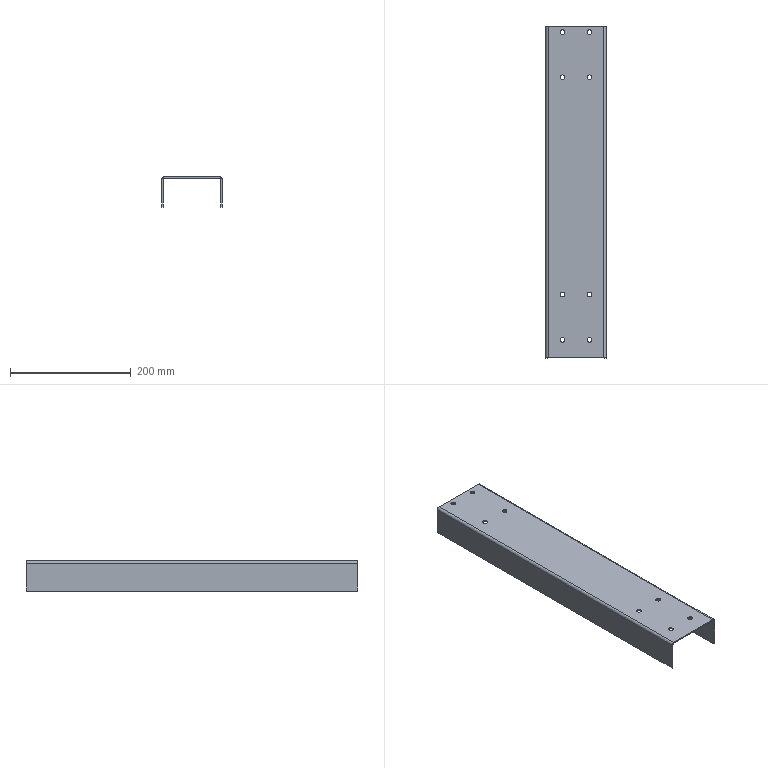Part | SolidWorks | features EdgeFlange 1, FlatPattern 1, ICE 1, SMBaseFlange 1, SheetMetal 1 | 1 solid | 38 faces | box 100 x 550 x 50 mm | volume 211963 mm3 | cylinder 20 | plane 18 | commonest cylinder face diameters 8 x18 4 x2
STEP:
#1=CARTESIAN_POINT('',(12.564,-446.02,-2.));
#2=VERTEX_POINT('',#1);
#3=CARTESIAN_POINT('',(20.564,-446.02,-2.));
#4=VERTEX_POINT('',#3);
#5=CARTESIAN_POINT('',(16.564,-446.02,-2.));
#6=DIRECTION('',(0.,0.,1.));
#7=DIRECTION('',(1.,0.,0.));
#8=AXIS2_PLACEMENT_3D('',#5,#6,#7);
#9=CIRCLE('',#8,4.);
#10=EDGE_CURVE('',#2,#4,#9,.T.);
#11=ORIENTED_EDGE('',*,*,#10,.F.);
#12=CARTESIAN_POINT('',(12.564,-446.02,0.));
#13=VERTEX_POINT('',#12);
#14=CARTESIAN_POINT('',(12.564,-446.02,-10.));
#15=DIRECTION('',(0.,0.,1.));
#16=VECTOR('',#15,1000.);
#17=LINE('',#14,#16);
#18=EDGE_CURVE('',#2,#13,#17,.T.);
#19=ORIENTED_EDGE('',*,*,#18,.T.);
#20=CARTESIAN_POINT('',(20.564,-446.02,0.));
#21=VERTEX_POINT('',#20);
#22=CARTESIAN_POINT('',(16.564,-446.02,0.));
#23=DIRECTION('',(0.,0.,1.));
#24=DIRECTION('',(-1.,0.,0.));
#25=AXIS2_PLACEMENT_3D('',#22,#23,#24);
#26=CIRCLE('',#25,4.);
#27=EDGE_CURVE('',#13,#21,#26,.T.);
#28=ORIENTED_EDGE('',*,*,#27,.T.);
#29=CARTESIAN_POINT('',(20.564,-446.02,-10.));
#30=DIRECTION('',(0.,0.,1.));
#31=VECTOR('',#30,1000.);
#32=LINE('',#29,#31);
#33=EDGE_CURVE('',#4,#21,#32,.T.);
#34=ORIENTED_EDGE('',*,*,#33,.F.);
#35=EDGE_LOOP('',(#11,#19,#28,#34));
#36=FACE_OUTER_BOUND('',#35,.T.);
#37=CARTESIAN_POINT('',(16.564,-446.02,-10.));
#38=DIRECTION('',(0.,0.,1.));
#39=DIRECTION('',(1.,0.,0.));
#40=AXIS2_PLACEMENT_3D('',#37,#38,#39);
#41=CYLINDRICAL_SURFACE('',#40,4.);
#42=ADVANCED_FACE('',(#36),#41,.F.);
#43=CARTESIAN_POINT('',(57.564,-446.02,-2.));
#44=VERTEX_POINT('',#43);
#45=CARTESIAN_POINT('',(65.564,-446.02,-2.));
#46=VERTEX_POINT('',#45);
#47=CARTESIAN_POINT('',(61.564,-446.02,-2.));
#48=DIRECTION('',(0.,0.,1.));
#49=DIRECTION('',(1.,0.,0.));
#50=AXIS2_PLACEMENT_3D('',#47,#48,#49);
#51=CIRCLE('',#50,4.);
#52=EDGE_CURVE('',#44,#46,#51,.T.);
#53=ORIENTED_EDGE('',*,*,#52,.F.);
#54=CARTESIAN_POINT('',(57.564,-446.02,0.));
#55=VERTEX_POINT('',#54);
#56=CARTESIAN_POINT('',(57.564,-446.02,-10.));
#57=DIRECTION('',(0.,0.,1.));
#58=VECTOR('',#57,1000.);
#59=LINE('',#56,#58);
#60=EDGE_CURVE('',#44,#55,#59,.T.);
#61=ORIENTED_EDGE('',*,*,#60,.T.);
#62=CARTESIAN_POINT('',(65.564,-446.02,0.));
#63=VERTEX_POINT('',#62);
#64=CARTESIAN_POINT('',(61.564,-446.02,0.));
#65=DIRECTION('',(0.,0.,1.));
#66=DIRECTION('',(-1.,0.,0.));
#67=AXIS2_PLACEMENT_3D('',#64,#65,#66);
#68=CIRCLE('',#67,4.);
#69=EDGE_CURVE('',#55,#63,#68,.T.);
#70=ORIENTED_EDGE('',*,*,#69,.T.);
#71=CARTESIAN_POINT('',(65.564,-446.02,-10.));
#72=DIRECTION('',(0.,0.,1.));
#73=VECTOR('',#72,1000.);
#74=LINE('',#71,#73);
#75=EDGE_CURVE('',#46,#63,#74,.T.);
#76=ORIENTED_EDGE('',*,*,#75,.F.);
#77=EDGE_LOOP('',(#53,#61,#70,#76));
#78=FACE_OUTER_BOUND('',#77,.T.);
#79=CARTESIAN_POINT('',(61.564,-446.02,-10.));
#80=DIRECTION('',(0.,0.,1.));
#81=DIRECTION('',(1.,0.,0.));
#82=AXIS2_PLACEMENT_3D('',#79,#80,#81);
#83=CYLINDRICAL_SURFACE('',#82,4.);
#84=ADVANCED_FACE('',(#78),#83,.F.);
#85=CARTESIAN_POINT('',(12.564,-371.02,-2.));
#86=VERTEX_POINT('',#85);
#87=CARTESIAN_POINT('',(20.564,-371.02,-2.));
#88=VERTEX_POINT('',#87);
#89=CARTESIAN_POINT('',(16.564,-371.02,-2.));
#90=DIRECTION('',(0.,0.,1.));
#91=DIRECTION('',(1.,0.,0.));
#92=AXIS2_PLACEMENT_3D('',#89,#90,#91);
#93=CIRCLE('',#92,4.);
#94=EDGE_CURVE('',#86,#88,#93,.T.);
#95=ORIENTED_EDGE('',*,*,#94,.F.);
#96=CARTESIAN_POINT('',(12.564,-371.02,0.));
#97=VERTEX_POINT('',#96);
#98=CARTESIAN_POINT('',(12.564,-371.02,-10.));
#99=DIRECTION('',(0.,0.,1.));
#100=VECTOR('',#99,1000.);
#101=LINE('',#98,#100);
#102=EDGE_CURVE('',#86,#97,#101,.T.);
#103=ORIENTED_EDGE('',*,*,#102,.T.);
#104=CARTESIAN_POINT('',(20.564,-371.02,0.));
#105=VERTEX_POINT('',#104);
#106=CARTESIAN_POINT('',(16.564,-371.02,0.));
#107=DIRECTION('',(0.,0.,1.));
#108=DIRECTION('',(-1.,0.,0.));
#109=AXIS2_PLACEMENT_3D('',#106,#107,#108);
#110=CIRCLE('',#109,4.);
#111=EDGE_CURVE('',#97,#105,#110,.T.);
#112=ORIENTED_EDGE('',*,*,#111,.T.);
#113=CARTESIAN_POINT('',(20.564,-371.02,-10.));
#114=DIRECTION('',(0.,0.,1.));
#115=VECTOR('',#114,1000.);
#116=LINE('',#113,#115);
#117=EDGE_CURVE('',#88,#105,#116,.T.);
#118=ORIENTED_EDGE('',*,*,#117,.F.);
#119=EDGE_LOOP('',(#95,#103,#112,#118));
#120=FACE_OUTER_BOUND('',#119,.T.);
#121=CARTESIAN_POINT('',(16.564,-371.02,-10.));
#122=DIRECTION('',(0.,0.,1.));
#123=DIRECTION('',(1.,0.,0.));
#124=AXIS2_PLACEMENT_3D('',#121,#122,#123);
#125=CYLINDRICAL_SURFACE('',#124,4.);
#126=ADVANCED_FACE('',(#120),#125,.F.);
#127=CARTESIAN_POINT('',(57.564,-371.02,-2.));
#128=VERTEX_POINT('',#127);
#129=CARTESIAN_POINT('',(65.564,-371.02,-2.));
#130=VERTEX_POINT('',#129);
#131=CARTESIAN_POINT('',(61.564,-371.02,-2.));
#132=DIRECTION('',(0.,0.,1.));
#133=DIRECTION('',(1.,0.,0.));
#134=AXIS2_PLACEMENT_3D('',#131,#132,#133);
#135=CIRCLE('',#134,4.);
#136=EDGE_CURVE('',#128,#130,#135,.T.);
#137=ORIENTED_EDGE('',*,*,#136,.F.);
#138=CARTESIAN_POINT('',(57.564,-371.02,0.));
#139=VERTEX_POINT('',#138);
#140=CARTESIAN_POINT('',(57.564,-371.02,-10.));
#141=DIRECTION('',(0.,0.,1.));
#142=VECTOR('',#141,1000.);
#143=LINE('',#140,#142);
#144=EDGE_CURVE('',#128,#139,#143,.T.);
#145=ORIENTED_EDGE('',*,*,#144,.T.);
#146=CARTESIAN_POINT('',(65.564,-371.02,0.));
#147=VERTEX_POINT('',#146);
#148=CARTESIAN_POINT('',(61.564,-371.02,0.));
#149=DIRECTION('',(0.,0.,1.));
#150=DIRECTION('',(-1.,0.,0.));
#151=AXIS2_PLACEMENT_3D('',#148,#149,#150);
#152=CIRCLE('',#151,4.);
#153=EDGE_CURVE('',#139,#147,#152,.T.);
#154=ORIENTED_EDGE('',*,*,#153,.T.);
#155=CARTESIAN_POINT('',(65.564,-371.02,-10.));
#156=DIRECTION('',(0.,0.,1.));
#157=VECTOR('',#156,1000.);
#158=LINE('',#155,#157);
#159=EDGE_CURVE('',#130,#147,#158,.T.);
#160=ORIENTED_EDGE('',*,*,#159,.F.);
#161=EDGE_LOOP('',(#137,#145,#154,#160));
#162=FACE_OUTER_BOUND('',#161,.T.);
#163=CARTESIAN_POINT('',(61.564,-371.02,-10.));
#164=DIRECTION('',(0.,0.,1.));
#165=DIRECTION('',(1.,0.,0.));
#166=AXIS2_PLACEMENT_3D('',#163,#164,#165);
#167=CYLINDRICAL_SURFACE('',#166,4.);
#168=ADVANCED_FACE('',(#162),#167,.F.);
#169=CARTESIAN_POINT('',(57.564,-11.02,-2.));
#170=VERTEX_POINT('',#169);
#171=CARTESIAN_POINT('',(65.564,-11.02,-2.));
#172=VERTEX_POINT('',#171);
#173=CARTESIAN_POINT('',(61.564,-11.02,-2.));
#174=DIRECTION('',(0.,0.,1.));
#175=DIRECTION('',(1.,0.,0.));
#176=AXIS2_PLACEMENT_3D('',#173,#174,#175);
#177=CIRCLE('',#176,4.);
#178=EDGE_CURVE('',#170,#172,#177,.T.);
#179=ORIENTED_EDGE('',*,*,#178,.F.);
#180=CARTESIAN_POINT('',(57.564,-11.02,0.));
#181=VERTEX_POINT('',#180);
#182=CARTESIAN_POINT('',(57.564,-11.02,-10.));
#183=DIRECTION('',(0.,0.,1.));
#184=VECTOR('',#183,1000.);
#185=LINE('',#182,#184);
#186=EDGE_CURVE('',#170,#181,#185,.T.);
#187=ORIENTED_EDGE('',*,*,#186,.T.);
#188=CARTESIAN_POINT('',(65.564,-11.02,0.));
#189=VERTEX_POINT('',#188);
#190=CARTESIAN_POINT('',(61.564,-11.02,0.));
#191=DIRECTION('',(0.,0.,1.));
#192=DIRECTION('',(1.,0.,0.));
#193=AXIS2_PLACEMENT_3D('',#190,#191,#192);
#194=CIRCLE('',#193,4.);
#195=EDGE_CURVE('',#181,#189,#194,.T.);
#196=ORIENTED_EDGE('',*,*,#195,.T.);
#197=CARTESIAN_POINT('',(65.564,-11.02,-10.));
#198=DIRECTION('',(0.,0.,1.));
#199=VECTOR('',#198,1000.);
#200=LINE('',#197,#199);
#201=EDGE_CURVE('',#172,#189,#200,.T.);
#202=ORIENTED_EDGE('',*,*,#201,.F.);
#203=EDGE_LOOP('',(#179,#187,#196,#202));
#204=FACE_OUTER_BOUND('',#203,.T.);
#205=CARTESIAN_POINT('',(61.564,-11.02,-10.));
#206=DIRECTION('',(0.,0.,1.));
#207=DIRECTION('',(1.,0.,0.));
#208=AXIS2_PLACEMENT_3D('',#205,#206,#207);
#209=CYLINDRICAL_SURFACE('',#208,4.);
#210=ADVANCED_FACE('',(#204),#209,.F.);
#211=CARTESIAN_POINT('',(12.564,-11.02,-2.));
#212=VERTEX_POINT('',#211);
#213=CARTESIAN_POINT('',(20.564,-11.02,-2.));
#214=VERTEX_POINT('',#213);
#215=CARTESIAN_POINT('',(16.564,-11.02,-2.));
#216=DIRECTION('',(0.,0.,1.));
#217=DIRECTION('',(1.,0.,0.));
#218=AXIS2_PLACEMENT_3D('',#215,#216,#217);
#219=CIRCLE('',#218,4.);
#220=EDGE_CURVE('',#212,#214,#219,.T.);
#221=ORIENTED_EDGE('',*,*,#220,.F.);
#222=CARTESIAN_POINT('',(12.564,-11.02,0.));
#223=VERTEX_POINT('',#222);
#224=CARTESIAN_POINT('',(12.564,-11.02,-10.));
#225=DIRECTION('',(0.,0.,1.));
#226=VECTOR('',#225,1000.);
#227=LINE('',#224,#226);
#228=EDGE_CURVE('',#212,#223,#227,.T.);
#229=ORIENTED_EDGE('',*,*,#228,.T.);
#230=CARTESIAN_POINT('',(20.564,-11.02,0.));
#231=VERTEX_POINT('',#230);
#232=CARTESIAN_POINT('',(16.564,-11.02,0.));
#233=DIRECTION('',(0.,0.,1.));
#234=DIRECTION('',(1.,0.,0.));
#235=AXIS2_PLACEMENT_3D('',#232,#233,#234);
#236=CIRCLE('',#235,4.);
#237=EDGE_CURVE('',#223,#231,#236,.T.);
#238=ORIENTED_EDGE('',*,*,#237,.T.);
#239=CARTESIAN_POINT('',(20.564,-11.02,-10.));
#240=DIRECTION('',(0.,0.,1.));
#241=VECTOR('',#240,1000.);
#242=LINE('',#239,#241);
#243=EDGE_CURVE('',#214,#231,#242,.T.);
#244=ORIENTED_EDGE('',*,*,#243,.F.);
#245=EDGE_LOOP('',(#221,#229,#238,#244));
#246=FACE_OUTER_BOUND('',#245,.T.);
#247=CARTESIAN_POINT('',(16.564,-11.02,-10.));
#248=DIRECTION('',(0.,0.,1.));
#249=DIRECTION('',(1.,0.,0.));
#250=AXIS2_PLACEMENT_3D('',#247,#248,#249);
#251=CYLINDRICAL_SURFACE('',#250,4.);
#252=ADVANCED_FACE('',(#246),#251,.F.);
#253=CARTESIAN_POINT('',(57.564,63.98,-2.));
#254=VERTEX_POINT('',#253);
#255=CARTESIAN_POINT('',(65.564,63.98,-2.));
#256=VERTEX_POINT('',#255);
#257=CARTESIAN_POINT('',(61.564,63.98,-2.));
#258=DIRECTION('',(0.,0.,1.));
#259=DIRECTION('',(1.,0.,0.));
#260=AXIS2_PLACEMENT_3D('',#257,#258,#259);
#261=CIRCLE('',#260,4.);
#262=EDGE_CURVE('',#254,#256,#261,.T.);
#263=ORIENTED_EDGE('',*,*,#262,.F.);
#264=CARTESIAN_POINT('',(57.564,63.98,0.));
#265=VERTEX_POINT('',#264);
#266=CARTESIAN_POINT('',(57.564,63.98,-10.));
#267=DIRECTION('',(0.,0.,1.));
#268=VECTOR('',#267,1000.);
#269=LINE('',#266,#268);
#270=EDGE_CURVE('',#254,#265,#269,.T.);
#271=ORIENTED_EDGE('',*,*,#270,.T.);
#272=CARTESIAN_POINT('',(65.564,63.98,0.));
#273=VERTEX_POINT('',#272);
#274=CARTESIAN_POINT('',(61.564,63.98,0.));
#275=DIRECTION('',(0.,0.,1.));
#276=DIRECTION('',(1.,0.,0.));
#277=AXIS2_PLACEMENT_3D('',#274,#275,#276);
#278=CIRCLE('',#277,4.);
#279=EDGE_CURVE('',#265,#273,#278,.T.);
#280=ORIENTED_EDGE('',*,*,#279,.T.);
#281=CARTESIAN_POINT('',(65.564,63.98,-10.));
#282=DIRECTION('',(0.,0.,1.));
#283=VECTOR('',#282,1000.);
#284=LINE('',#281,#283);
#285=EDGE_CURVE('',#256,#273,#284,.T.);
#286=ORIENTED_EDGE('',*,*,#285,.F.);
#287=EDGE_LOOP('',(#263,#271,#280,#286));
#288=FACE_OUTER_BOUND('',#287,.T.);
#289=CARTESIAN_POINT('',(61.564,63.98,-10.));
#290=DIRECTION('',(0.,0.,1.));
#291=DIRECTION('',(1.,0.,0.));
#292=AXIS2_PLACEMENT_3D('',#289,#290,#291);
#293=CYLINDRICAL_SURFACE('',#292,4.);
#294=ADVANCED_FACE('',(#288),#293,.F.);
#295=CARTESIAN_POINT('',(12.564,63.98,-2.));
#296=VERTEX_POINT('',#295);
#297=CARTESIAN_POINT('',(20.564,63.98,-2.));
#298=VERTEX_POINT('',#297);
#299=CARTESIAN_POINT('',(16.564,63.98,-2.));
#300=DIRECTION('',(0.,0.,1.));
#301=DIRECTION('',(1.,0.,0.));
#302=AXIS2_PLACEMENT_3D('',#299,#300,#301);
#303=CIRCLE('',#302,4.);
#304=EDGE_CURVE('',#296,#298,#303,.T.);
#305=ORIENTED_EDGE('',*,*,#304,.F.);
#306=CARTESIAN_POINT('',(12.564,63.98,0.));
#307=VERTEX_POINT('',#306);
#308=CARTESIAN_POINT('',(12.564,63.98,-10.));
#309=DIRECTION('',(0.,0.,1.));
#310=VECTOR('',#309,1000.);
#311=LINE('',#308,#310);
#312=EDGE_CURVE('',#296,#307,#311,.T.);
#313=ORIENTED_EDGE('',*,*,#312,.T.);
#314=CARTESIAN_POINT('',(20.564,63.98,0.));
#315=VERTEX_POINT('',#314);
#316=CARTESIAN_POINT('',(16.564,63.98,0.));
#317=DIRECTION('',(0.,0.,1.));
#318=DIRECTION('',(1.,0.,0.));
#319=AXIS2_PLACEMENT_3D('',#316,#317,#318);
#320=CIRCLE('',#319,4.);
#321=EDGE_CURVE('',#307,#315,#320,.T.);
#322=ORIENTED_EDGE('',*,*,#321,.T.);
#323=CARTESIAN_POINT('',(20.564,63.98,-10.));
#324=DIRECTION('',(0.,0.,1.));
#325=VECTOR('',#324,1000.);
#326=LINE('',#323,#325);
#327=EDGE_CURVE('',#298,#315,#326,.T.);
#328=ORIENTED_EDGE('',*,*,#327,.F.);
#329=EDGE_LOOP('',(#305,#313,#322,#328));
#330=FACE_OUTER_BOUND('',#329,.T.);
#331=CARTESIAN_POINT('',(16.564,63.98,-10.));
#332=DIRECTION('',(0.,0.,1.));
#333=DIRECTION('',(1.,0.,0.));
#334=AXIS2_PLACEMENT_3D('',#331,#332,#333);
#335=CYLINDRICAL_SURFACE('',#334,4.);
#336=ADVANCED_FACE('',(#330),#335,.F.);
#337=CARTESIAN_POINT('',(16.564,-446.02,-2.));
#338=DIRECTION('',(0.,0.,1.));
#339=DIRECTION('',(1.,0.,0.));
#340=AXIS2_PLACEMENT_3D('',#337,#338,#339);
#341=CIRCLE('',#340,4.);
#342=EDGE_CURVE('',#4,#2,#341,.T.);
#343=ORIENTED_EDGE('',*,*,#342,.T.);
#344=ORIENTED_EDGE('',*,*,#10,.T.);
#345=EDGE_LOOP('',(#343,#344));
#346=FACE_BOUND('',#345,.T.);
#347=CARTESIAN_POINT('',(61.564,-446.02,-2.));
#348=DIRECTION('',(0.,0.,1.));
#349=DIRECTION('',(1.,0.,0.));
#350=AXIS2_PLACEMENT_3D('',#347,#348,#349);
#351=CIRCLE('',#350,4.);
#352=EDGE_CURVE('',#46,#44,#351,.T.);
#353=ORIENTED_EDGE('',*,*,#352,.T.);
#354=ORIENTED_EDGE('',*,*,#52,.T.);
#355=EDGE_LOOP('',(#353,#354));
#356=FACE_BOUND('',#355,.T.);
#357=CARTESIAN_POINT('',(16.564,-371.02,-2.));
#358=DIRECTION('',(0.,0.,1.));
#359=DIRECTION('',(1.,0.,0.));
#360=AXIS2_PLACEMENT_3D('',#357,#358,#359);
#361=CIRCLE('',#360,4.);
#362=EDGE_CURVE('',#88,#86,#361,.T.);
#363=ORIENTED_EDGE('',*,*,#362,.T.);
#364=ORIENTED_EDGE('',*,*,#94,.T.);
#365=EDGE_LOOP('',(#363,#364));
#366=FACE_BOUND('',#365,.T.);
#367=CARTESIAN_POINT('',(61.564,-371.02,-2.));
#368=DIRECTION('',(0.,0.,1.));
#369=DIRECTION('',(1.,0.,0.));
#370=AXIS2_PLACEMENT_3D('',#367,#368,#369);
#371=CIRCLE('',#370,4.);
#372=EDGE_CURVE('',#130,#128,#371,.T.);
#373=ORIENTED_EDGE('',*,*,#372,.T.);
#374=ORIENTED_EDGE('',*,*,#136,.T.);
#375=EDGE_LOOP('',(#373,#374));
#376=FACE_BOUND('',#375,.T.);
#377=CARTESIAN_POINT('',(61.564,-11.02,-2.));
#378=DIRECTION('',(0.,0.,1.));
#379=DIRECTION('',(1.,0.,0.));
#380=AXIS2_PLACEMENT_3D('',#377,#378,#379);
#381=CIRCLE('',#380,4.);
#382=EDGE_CURVE('',#172,#170,#381,.T.);
#383=ORIENTED_EDGE('',*,*,#382,.T.);
#384=ORIENTED_EDGE('',*,*,#178,.T.);
#385=EDGE_LOOP('',(#383,#384));
#386=FACE_BOUND('',#385,.T.);
#387=CARTESIAN_POINT('',(16.564,-11.02,-2.));
#388=DIRECTION('',(0.,0.,1.));
#389=DIRECTION('',(1.,0.,0.));
#390=AXIS2_PLACEMENT_3D('',#387,#388,#389);
#391=CIRCLE('',#390,4.);
#392=EDGE_CURVE('',#214,#212,#391,.T.);
#393=ORIENTED_EDGE('',*,*,#392,.T.);
#394=ORIENTED_EDGE('',*,*,#220,.T.);
#395=EDGE_LOOP('',(#393,#394));
#396=FACE_BOUND('',#395,.T.);
#397=CARTESIAN_POINT('',(61.564,63.98,-2.));
#398=DIRECTION('',(0.,0.,1.));
#399=DIRECTION('',(1.,0.,0.));
#400=AXIS2_PLACEMENT_3D('',#397,#398,#399);
#401=CIRCLE('',#400,4.);
#402=EDGE_CURVE('',#256,#254,#401,.T.);
#403=ORIENTED_EDGE('',*,*,#402,.T.);
#404=ORIENTED_EDGE('',*,*,#262,.T.);
#405=EDGE_LOOP('',(#403,#404));
#406=FACE_BOUND('',#405,.T.);
#407=CARTESIAN_POINT('',(16.564,63.98,-2.));
#408=DIRECTION('',(0.,0.,1.));
#409=DIRECTION('',(1.,0.,0.));
#410=AXIS2_PLACEMENT_3D('',#407,#408,#409);
#411=CIRCLE('',#410,4.);
#412=EDGE_CURVE('',#298,#296,#411,.T.);
#413=ORIENTED_EDGE('',*,*,#412,.T.);
#414=ORIENTED_EDGE('',*,*,#304,.T.);
#415=EDGE_LOOP('',(#413,#414));
#416=FACE_BOUND('',#415,.T.);
#417=CARTESIAN_POINT('',(85.064,-476.02,-2.));
#418=VERTEX_POINT('',#417);
#419=CARTESIAN_POINT('',(85.064,73.98,-2.));
#420=VERTEX_POINT('',#419);
#421=CARTESIAN_POINT('',(85.064,-476.02,-2.));
#422=DIRECTION('',(0.,1.,0.));
#423=VECTOR('',#422,1000.);
#424=LINE('',#421,#423);
#425=EDGE_CURVE('',#418,#420,#424,.T.);
#426=ORIENTED_EDGE('',*,*,#425,.F.);
#427=CARTESIAN_POINT('',(-6.936,-476.02,-2.));
#428=VERTEX_POINT('',#427);
#429=CARTESIAN_POINT('',(-10.936,-476.02,-2.));
#430=DIRECTION('',(1.,0.,0.));
#431=VECTOR('',#430,1000.);
#432=LINE('',#429,#431);
#433=EDGE_CURVE('',#428,#418,#432,.T.);
#434=ORIENTED_EDGE('',*,*,#433,.F.);
#435=CARTESIAN_POINT('',(-6.936,73.98,-2.));
#436=VERTEX_POINT('',#435);
#437=CARTESIAN_POINT('',(-6.936,73.98,-2.));
#438=DIRECTION('',(0.,-1.,0.));
#439=VECTOR('',#438,1000.);
#440=LINE('',#437,#439);
#441=EDGE_CURVE('',#436,#428,#440,.T.);
#442=ORIENTED_EDGE('',*,*,#441,.F.);
#443=CARTESIAN_POINT('',(-10.936,73.98,-2.));
#444=DIRECTION('',(-1.,0.,0.));
#445=VECTOR('',#444,1000.);
#446=LINE('',#443,#445);
#447=EDGE_CURVE('',#420,#436,#446,.T.);
#448=ORIENTED_EDGE('',*,*,#447,.F.);
#449=EDGE_LOOP('',(#426,#434,#442,#448));
#450=FACE_OUTER_BOUND('',#449,.T.);
#451=CARTESIAN_POINT('',(0.,0.,-2.));
#452=DIRECTION('',(0.,0.,1.));
#453=DIRECTION('',(1.,0.,0.));
#454=AXIS2_PLACEMENT_3D('',#451,#452,#453);
#455=PLANE('',#454);
#456=ADVANCED_FACE('',(#346,#356,#366,#376,#386,#396,#406,#416,#450),#455,.F.);
#457=CARTESIAN_POINT('',(16.564,-446.02,0.));
#458=DIRECTION('',(0.,0.,1.));
#459=DIRECTION('',(-1.,0.,0.));
#460=AXIS2_PLACEMENT_3D('',#457,#458,#459);
#461=CIRCLE('',#460,4.);
#462=EDGE_CURVE('',#21,#13,#461,.T.);
#463=ORIENTED_EDGE('',*,*,#462,.F.);
#464=ORIENTED_EDGE('',*,*,#27,.F.);
#465=EDGE_LOOP('',(#463,#464));
#466=FACE_BOUND('',#465,.T.);
#467=CARTESIAN_POINT('',(61.564,-446.02,0.));
#468=DIRECTION('',(0.,0.,1.));
#469=DIRECTION('',(-1.,0.,0.));
#470=AXIS2_PLACEMENT_3D('',#467,#468,#469);
#471=CIRCLE('',#470,4.);
#472=EDGE_CURVE('',#63,#55,#471,.T.);
#473=ORIENTED_EDGE('',*,*,#472,.F.);
#474=ORIENTED_EDGE('',*,*,#69,.F.);
#475=EDGE_LOOP('',(#473,#474));
#476=FACE_BOUND('',#475,.T.);
#477=CARTESIAN_POINT('',(16.564,-371.02,0.));
#478=DIRECTION('',(0.,0.,1.));
#479=DIRECTION('',(-1.,0.,0.));
#480=AXIS2_PLACEMENT_3D('',#477,#478,#479);
#481=CIRCLE('',#480,4.);
#482=EDGE_CURVE('',#105,#97,#481,.T.);
#483=ORIENTED_EDGE('',*,*,#482,.F.);
#484=ORIENTED_EDGE('',*,*,#111,.F.);
#485=EDGE_LOOP('',(#483,#484));
#486=FACE_BOUND('',#485,.T.);
#487=CARTESIAN_POINT('',(61.564,-371.02,0.));
#488=DIRECTION('',(0.,0.,1.));
#489=DIRECTION('',(-1.,0.,0.));
#490=AXIS2_PLACEMENT_3D('',#487,#488,#489);
#491=CIRCLE('',#490,4.);
#492=EDGE_CURVE('',#147,#139,#491,.T.);
#493=ORIENTED_EDGE('',*,*,#492,.F.);
#494=ORIENTED_EDGE('',*,*,#153,.F.);
#495=EDGE_LOOP('',(#493,#494));
#496=FACE_BOUND('',#495,.T.);
#497=CARTESIAN_POINT('',(61.564,-11.02,0.));
#498=DIRECTION('',(0.,0.,1.));
#499=DIRECTION('',(1.,0.,0.));
#500=AXIS2_PLACEMENT_3D('',#497,#498,#499);
#501=CIRCLE('',#500,4.);
#502=EDGE_CURVE('',#189,#181,#501,.T.);
#503=ORIENTED_EDGE('',*,*,#502,.F.);
#504=ORIENTED_EDGE('',*,*,#195,.F.);
#505=EDGE_LOOP('',(#503,#504));
#506=FACE_BOUND('',#505,.T.);
#507=CARTESIAN_POINT('',(16.564,-11.02,0.));
#508=DIRECTION('',(0.,0.,1.));
#509=DIRECTION('',(1.,0.,0.));
#510=AXIS2_PLACEMENT_3D('',#507,#508,#509);
#511=CIRCLE('',#510,4.);
#512=EDGE_CURVE('',#231,#223,#511,.T.);
#513=ORIENTED_EDGE('',*,*,#512,.F.);
#514=ORIENTED_EDGE('',*,*,#237,.F.);
#515=EDGE_LOOP('',(#513,#514));
#516=FACE_BOUND('',#515,.T.);
#517=CARTESIAN_POINT('',(61.564,63.98,0.));
#518=DIRECTION('',(0.,0.,1.));
#519=DIRECTION('',(1.,0.,0.));
#520=AXIS2_PLACEMENT_3D('',#517,#518,#519);
#521=CIRCLE('',#520,4.);
#522=EDGE_CURVE('',#273,#265,#521,.T.);
#523=ORIENTED_EDGE('',*,*,#522,.F.);
#524=ORIENTED_EDGE('',*,*,#279,.F.);
#525=EDGE_LOOP('',(#523,#524));
#526=FACE_BOUND('',#525,.T.);
#527=CARTESIAN_POINT('',(16.564,63.98,0.));
#528=DIRECTION('',(0.,0.,1.));
#529=DIRECTION('',(1.,0.,0.));
#530=AXIS2_PLACEMENT_3D('',#527,#528,#529);
#531=CIRCLE('',#530,4.);
#532=EDGE_CURVE('',#315,#307,#531,.T.);
#533=ORIENTED_EDGE('',*,*,#532,.F.);
#534=ORIENTED_EDGE('',*,*,#321,.F.);
#535=EDGE_LOOP('',(#533,#534));
#536=FACE_BOUND('',#535,.T.);
#537=CARTESIAN_POINT('',(-6.936,-476.02,0.));
#538=VERTEX_POINT('',#537);
#539=CARTESIAN_POINT('',(85.064,-476.02,0.));
#540=VERTEX_POINT('',#539);
#541=CARTESIAN_POINT('',(-10.936,-476.02,0.));
#542=DIRECTION('',(1.,0.,0.));
#543=VECTOR('',#542,1000.);
#544=LINE('',#541,#543);
#545=EDGE_CURVE('',#538,#540,#544,.T.);
#546=ORIENTED_EDGE('',*,*,#545,.T.);
#547=CARTESIAN_POINT('',(85.064,73.98,0.));
#548=VERTEX_POINT('',#547);
#549=CARTESIAN_POINT('',(85.064,-476.02,0.));
#550=DIRECTION('',(0.,1.,0.));
#551=VECTOR('',#550,1000.);
#552=LINE('',#549,#551);
#553=EDGE_CURVE('',#540,#548,#552,.T.);
#554=ORIENTED_EDGE('',*,*,#553,.T.);
#555=CARTESIAN_POINT('',(-6.936,73.98,0.));
#556=VERTEX_POINT('',#555);
#557=CARTESIAN_POINT('',(-10.936,73.98,0.));
#558=DIRECTION('',(-1.,0.,0.));
#559=VECTOR('',#558,1000.);
#560=LINE('',#557,#559);
#561=EDGE_CURVE('',#548,#556,#560,.T.);
#562=ORIENTED_EDGE('',*,*,#561,.T.);
#563=CARTESIAN_POINT('',(-6.936,73.98,0.));
#564=DIRECTION('',(0.,-1.,0.));
#565=VECTOR('',#564,1000.);
#566=LINE('',#563,#565);
#567=EDGE_CURVE('',#556,#538,#566,.T.);
#568=ORIENTED_EDGE('',*,*,#567,.T.);
#569=EDGE_LOOP('',(#546,#554,#562,#568));
#570=FACE_OUTER_BOUND('',#569,.T.);
#571=CARTESIAN_POINT('',(0.,0.,0.));
#572=DIRECTION('',(0.,0.,1.));
#573=DIRECTION('',(1.,0.,0.));
#574=AXIS2_PLACEMENT_3D('',#571,#572,#573);
#575=PLANE('',#574);
#576=ADVANCED_FACE('',(#466,#476,#486,#496,#506,#516,#526,#536,#570),#575,.T.);
#577=ORIENTED_EDGE('',*,*,#433,.T.);
#578=CARTESIAN_POINT('',(85.064,-476.02,-2.));
#579=DIRECTION('',(0.,0.,1.));
#580=VECTOR('',#579,1000.);
#581=LINE('',#578,#580);
#582=EDGE_CURVE('',#418,#540,#581,.T.);
#583=ORIENTED_EDGE('',*,*,#582,.T.);
#584=ORIENTED_EDGE('',*,*,#545,.F.);
#585=CARTESIAN_POINT('',(-6.936,-476.02,-2.));
#586=DIRECTION('',(0.,0.,1.));
#587=VECTOR('',#586,1000.);
#588=LINE('',#585,#587);
#589=EDGE_CURVE('',#428,#538,#588,.T.);
#590=ORIENTED_EDGE('',*,*,#589,.F.);
#591=EDGE_LOOP('',(#577,#583,#584,#590));
#592=FACE_OUTER_BOUND('',#591,.T.);
#593=CARTESIAN_POINT('',(-10.936,-476.02,-2.));
#594=DIRECTION('',(0.,-1.,0.));
#595=DIRECTION('',(0.,0.,-1.));
#596=AXIS2_PLACEMENT_3D('',#593,#594,#595);
#597=PLANE('',#596);
#598=ADVANCED_FACE('',(#592),#597,.T.);
#599=CARTESIAN_POINT('',(85.064,73.98,-2.));
#600=DIRECTION('',(0.,0.,1.));
#601=VECTOR('',#600,1000.);
#602=LINE('',#599,#601);
#603=EDGE_CURVE('',#420,#548,#602,.T.);
#604=ORIENTED_EDGE('',*,*,#603,.F.);
#605=ORIENTED_EDGE('',*,*,#447,.T.);
#606=CARTESIAN_POINT('',(-6.936,73.98,-2.));
#607=DIRECTION('',(0.,0.,1.));
#608=VECTOR('',#607,1000.);
#609=LINE('',#606,#608);
#610=EDGE_CURVE('',#436,#556,#609,.T.);
#611=ORIENTED_EDGE('',*,*,#610,.T.);
#612=ORIENTED_EDGE('',*,*,#561,.F.);
#613=EDGE_LOOP('',(#604,#605,#611,#612));
#614=FACE_OUTER_BOUND('',#613,.T.);
#615=CARTESIAN_POINT('',(-10.936,73.98,-2.));
#616=DIRECTION('',(0.,1.,0.));
#617=DIRECTION('',(0.,0.,1.));
#618=AXIS2_PLACEMENT_3D('',#615,#616,#617);
#619=PLANE('',#618);
#620=ADVANCED_FACE('',(#614),#619,.T.);
#621=CARTESIAN_POINT('',(-8.936,-476.02,-4.));
#622=VERTEX_POINT('',#621);
#623=CARTESIAN_POINT('',(-10.936,-476.02,-4.));
#624=VERTEX_POINT('',#623);
#625=CARTESIAN_POINT('',(-10.936,-476.02,-4.));
#626=DIRECTION('',(-1.,0.,0.));
#627=VECTOR('',#626,1000.);
#628=LINE('',#625,#627);
#629=EDGE_CURVE('',#622,#624,#628,.T.);
#630=ORIENTED_EDGE('',*,*,#629,.F.);
#631=CARTESIAN_POINT('',(-6.936,-476.02,-4.));
#632=DIRECTION('',(0.,-1.,0.));
#633=DIRECTION('',(-1.,0.,0.));
#634=AXIS2_PLACEMENT_3D('',#631,#632,#633);
#635=CIRCLE('',#634,2.);
#636=EDGE_CURVE('',#428,#622,#635,.T.);
#637=ORIENTED_EDGE('',*,*,#636,.F.);
#638=ORIENTED_EDGE('',*,*,#589,.T.);
#639=CARTESIAN_POINT('',(-6.936,-476.02,-4.));
#640=DIRECTION('',(0.,-1.,0.));
#641=DIRECTION('',(-1.,0.,0.));
#642=AXIS2_PLACEMENT_3D('',#639,#640,#641);
#643=CIRCLE('',#642,4.);
#644=EDGE_CURVE('',#538,#624,#643,.T.);
#645=ORIENTED_EDGE('',*,*,#644,.T.);
#646=EDGE_LOOP('',(#630,#637,#638,#645));
#647=FACE_OUTER_BOUND('',#646,.T.);
#648=CARTESIAN_POINT('',(-6.936,-476.02,-4.));
#649=DIRECTION('',(0.,-1.,0.));
#650=DIRECTION('',(1.,0.,0.));
#651=AXIS2_PLACEMENT_3D('',#648,#649,#650);
#652=PLANE('',#651);
#653=ADVANCED_FACE('',(#647),#652,.T.);
#654=CARTESIAN_POINT('',(-8.936,73.98,-4.));
#655=VERTEX_POINT('',#654);
#656=CARTESIAN_POINT('',(-6.936,73.98,-4.));
#657=DIRECTION('',(0.,1.,0.));
#658=DIRECTION('',(-1.,0.,0.));
#659=AXIS2_PLACEMENT_3D('',#656,#657,#658);
#660=CIRCLE('',#659,2.);
#661=EDGE_CURVE('',#655,#436,#660,.T.);
#662=ORIENTED_EDGE('',*,*,#661,.F.);
#663=CARTESIAN_POINT('',(-10.936,73.98,-4.));
#664=VERTEX_POINT('',#663);
#665=CARTESIAN_POINT('',(-8.936,73.98,-4.));
#666=DIRECTION('',(-1.,0.,0.));
#667=VECTOR('',#666,1000.);
#668=LINE('',#665,#667);
#669=EDGE_CURVE('',#655,#664,#668,.T.);
#670=ORIENTED_EDGE('',*,*,#669,.T.);
#671=CARTESIAN_POINT('',(-6.936,73.98,-4.));
#672=DIRECTION('',(0.,1.,0.));
#673=DIRECTION('',(-1.,0.,0.));
#674=AXIS2_PLACEMENT_3D('',#671,#672,#673);
#675=CIRCLE('',#674,4.);
#676=EDGE_CURVE('',#664,#556,#675,.T.);
#677=ORIENTED_EDGE('',*,*,#676,.T.);
#678=ORIENTED_EDGE('',*,*,#610,.F.);
#679=EDGE_LOOP('',(#662,#670,#677,#678));
#680=FACE_OUTER_BOUND('',#679,.T.);
#681=CARTESIAN_POINT('',(-6.936,73.98,-4.));
#682=DIRECTION('',(0.,-1.,0.));
#683=DIRECTION('',(1.,0.,0.));
#684=AXIS2_PLACEMENT_3D('',#681,#682,#683);
#685=PLANE('',#684);
#686=ADVANCED_FACE('',(#680),#685,.F.);
#687=ORIENTED_EDGE('',*,*,#567,.F.);
#688=ORIENTED_EDGE('',*,*,#676,.F.);
#689=CARTESIAN_POINT('',(-10.936,0.,-4.));
#690=DIRECTION('',(0.,1.,0.));
#691=VECTOR('',#690,1000.);
#692=LINE('',#689,#691);
#693=EDGE_CURVE('',#624,#664,#692,.T.);
#694=ORIENTED_EDGE('',*,*,#693,.F.);
#695=ORIENTED_EDGE('',*,*,#644,.F.);
#696=EDGE_LOOP('',(#687,#688,#694,#695));
#697=FACE_OUTER_BOUND('',#696,.T.);
#698=CARTESIAN_POINT('',(-6.936,73.98,-4.));
#699=DIRECTION('',(0.,1.,0.));
#700=DIRECTION('',(-1.,0.,0.));
#701=AXIS2_PLACEMENT_3D('',#698,#699,#700);
#702=CYLINDRICAL_SURFACE('',#701,4.);
#703=ADVANCED_FACE('',(#697),#702,.T.);
#704=ORIENTED_EDGE('',*,*,#441,.T.);
#705=ORIENTED_EDGE('',*,*,#636,.T.);
#706=CARTESIAN_POINT('',(-8.936,-476.02,-4.));
#707=DIRECTION('',(0.,1.,0.));
#708=VECTOR('',#707,1000.);
#709=LINE('',#706,#708);
#710=EDGE_CURVE('',#622,#655,#709,.T.);
#711=ORIENTED_EDGE('',*,*,#710,.T.);
#712=ORIENTED_EDGE('',*,*,#661,.T.);
#713=EDGE_LOOP('',(#704,#705,#711,#712));
#714=FACE_OUTER_BOUND('',#713,.T.);
#715=CARTESIAN_POINT('',(-6.936,73.98,-4.));
#716=DIRECTION('',(0.,1.,0.));
#717=DIRECTION('',(-1.,0.,0.));
#718=AXIS2_PLACEMENT_3D('',#715,#716,#717);
#719=CYLINDRICAL_SURFACE('',#718,2.);
#720=ADVANCED_FACE('',(#714),#719,.F.);
#721=CARTESIAN_POINT('',(-10.936,73.98,-50.));
#722=VERTEX_POINT('',#721);
#723=CARTESIAN_POINT('',(-10.936,73.98,-2.));
#724=DIRECTION('',(0.,0.,1.));
#725=VECTOR('',#724,1000.);
#726=LINE('',#723,#725);
#727=EDGE_CURVE('',#722,#664,#726,.T.);
#728=ORIENTED_EDGE('',*,*,#727,.T.);
#729=ORIENTED_EDGE('',*,*,#669,.F.);
#730=CARTESIAN_POINT('',(-8.936,73.98,-50.));
#731=VERTEX_POINT('',#730);
#732=CARTESIAN_POINT('',(-8.936,73.98,0.));
#733=DIRECTION('',(0.,0.,1.));
#734=VECTOR('',#733,1000.);
#735=LINE('',#732,#734);
#736=EDGE_CURVE('',#731,#655,#735,.T.);
#737=ORIENTED_EDGE('',*,*,#736,.F.);
#738=CARTESIAN_POINT('',(-10.936,73.98,-50.));
#739=DIRECTION('',(1.,0.,0.));
#740=VECTOR('',#739,1000.);
#741=LINE('',#738,#740);
#742=EDGE_CURVE('',#722,#731,#741,.T.);
#743=ORIENTED_EDGE('',*,*,#742,.F.);
#744=EDGE_LOOP('',(#728,#729,#737,#743));
#745=FACE_OUTER_BOUND('',#744,.T.);
#746=CARTESIAN_POINT('',(-10.936,73.98,-2.));
#747=DIRECTION('',(0.,1.,0.));
#748=DIRECTION('',(-1.,0.,0.));
#749=AXIS2_PLACEMENT_3D('',#746,#747,#748);
#750=PLANE('',#749);
#751=ADVANCED_FACE('',(#745),#750,.T.);
#752=CARTESIAN_POINT('',(-8.936,-476.02,-50.));
#753=VERTEX_POINT('',#752);
#754=CARTESIAN_POINT('',(-8.936,-476.02,0.));
#755=DIRECTION('',(0.,0.,-1.));
#756=VECTOR('',#755,1000.);
#757=LINE('',#754,#756);
#758=EDGE_CURVE('',#622,#753,#757,.T.);
#759=ORIENTED_EDGE('',*,*,#758,.F.);
#760=ORIENTED_EDGE('',*,*,#629,.T.);
#761=CARTESIAN_POINT('',(-10.936,-476.02,-50.));
#762=VERTEX_POINT('',#761);
#763=CARTESIAN_POINT('',(-10.936,-476.02,-50.));
#764=DIRECTION('',(0.,0.,-1.));
#765=VECTOR('',#764,1000.);
#766=LINE('',#763,#765);
#767=EDGE_CURVE('',#624,#762,#766,.T.);
#768=ORIENTED_EDGE('',*,*,#767,.T.);
#769=CARTESIAN_POINT('',(-10.936,-476.02,-50.));
#770=DIRECTION('',(1.,0.,0.));
#771=VECTOR('',#770,1000.);
#772=LINE('',#769,#771);
#773=EDGE_CURVE('',#762,#753,#772,.T.);
#774=ORIENTED_EDGE('',*,*,#773,.T.);
#775=EDGE_LOOP('',(#759,#760,#768,#774));
#776=FACE_OUTER_BOUND('',#775,.T.);
#777=CARTESIAN_POINT('',(-10.936,-476.02,-50.));
#778=DIRECTION('',(0.,-1.,0.));
#779=DIRECTION('',(1.,0.,0.));
#780=AXIS2_PLACEMENT_3D('',#777,#778,#779);
#781=PLANE('',#780);
#782=ADVANCED_FACE('',(#776),#781,.T.);
#783=ORIENTED_EDGE('',*,*,#767,.F.);
#784=ORIENTED_EDGE('',*,*,#693,.T.);
#785=ORIENTED_EDGE('',*,*,#727,.F.);
#786=CARTESIAN_POINT('',(-10.936,73.98,-50.));
#787=DIRECTION('',(0.,1.,0.));
#788=VECTOR('',#787,1000.);
#789=LINE('',#786,#788);
#790=EDGE_CURVE('',#762,#722,#789,.T.);
#791=ORIENTED_EDGE('',*,*,#790,.F.);
#792=EDGE_LOOP('',(#783,#784,#785,#791));
#793=FACE_OUTER_BOUND('',#792,.T.);
#794=CARTESIAN_POINT('',(-10.936,0.,0.));
#795=DIRECTION('',(-1.,0.,0.));
#796=DIRECTION('',(0.,0.,1.));
#797=AXIS2_PLACEMENT_3D('',#794,#795,#796);
#798=PLANE('',#797);
#799=ADVANCED_FACE('',(#793),#798,.T.);
#800=ORIENTED_EDGE('',*,*,#710,.F.);
#801=ORIENTED_EDGE('',*,*,#758,.T.);
#802=CARTESIAN_POINT('',(-8.936,0.,-50.));
#803=DIRECTION('',(0.,1.,0.));
#804=VECTOR('',#803,1000.);
#805=LINE('',#802,#804);
#806=EDGE_CURVE('',#753,#731,#805,.T.);
#807=ORIENTED_EDGE('',*,*,#806,.T.);
#808=ORIENTED_EDGE('',*,*,#736,.T.);
#809=EDGE_LOOP('',(#800,#801,#807,#808));
#810=FACE_OUTER_BOUND('',#809,.T.);
#811=CARTESIAN_POINT('',(-8.936,0.,0.));
#812=DIRECTION('',(-1.,0.,0.));
#813=DIRECTION('',(0.,0.,1.));
#814=AXIS2_PLACEMENT_3D('',#811,#812,#813);
#815=PLANE('',#814);
#816=ADVANCED_FACE('',(#810),#815,.F.);
#817=ORIENTED_EDGE('',*,*,#806,.F.);
#818=ORIENTED_EDGE('',*,*,#773,.F.);
#819=ORIENTED_EDGE('',*,*,#790,.T.);
#820=ORIENTED_EDGE('',*,*,#742,.T.);
#821=EDGE_LOOP('',(#817,#818,#819,#820));
#822=FACE_OUTER_BOUND('',#821,.T.);
#823=CARTESIAN_POINT('',(-10.936,73.98,-50.));
#824=DIRECTION('',(0.,0.,-1.));
#825=DIRECTION('',(-1.,0.,0.));
#826=AXIS2_PLACEMENT_3D('',#823,#824,#825);
#827=PLANE('',#826);
#828=ADVANCED_FACE('',(#822),#827,.T.);
#829=CARTESIAN_POINT('',(87.064,73.98,-4.));
#830=VERTEX_POINT('',#829);
#831=CARTESIAN_POINT('',(89.064,73.98,-4.));
#832=VERTEX_POINT('',#831);
#833=CARTESIAN_POINT('',(89.064,73.98,-4.));
#834=DIRECTION('',(1.,0.,0.));
#835=VECTOR('',#834,1000.);
#836=LINE('',#833,#835);
#837=EDGE_CURVE('',#830,#832,#836,.T.);
#838=ORIENTED_EDGE('',*,*,#837,.F.);
#839=CARTESIAN_POINT('',(85.064,73.98,-4.));
#840=DIRECTION('',(0.,1.,0.));
#841=DIRECTION('',(0.,0.,-1.));
#842=AXIS2_PLACEMENT_3D('',#839,#840,#841);
#843=CIRCLE('',#842,2.);
#844=EDGE_CURVE('',#420,#830,#843,.T.);
#845=ORIENTED_EDGE('',*,*,#844,.F.);
#846=ORIENTED_EDGE('',*,*,#603,.T.);
#847=CARTESIAN_POINT('',(85.064,73.98,-4.));
#848=DIRECTION('',(0.,1.,0.));
#849=DIRECTION('',(0.,0.,-1.));
#850=AXIS2_PLACEMENT_3D('',#847,#848,#849);
#851=CIRCLE('',#850,4.);
#852=EDGE_CURVE('',#548,#832,#851,.T.);
#853=ORIENTED_EDGE('',*,*,#852,.T.);
#854=EDGE_LOOP('',(#838,#845,#846,#853));
#855=FACE_OUTER_BOUND('',#854,.T.);
#856=CARTESIAN_POINT('',(85.064,73.98,-4.));
#857=DIRECTION('',(0.,1.,0.));
#858=DIRECTION('',(0.,0.,1.));
#859=AXIS2_PLACEMENT_3D('',#856,#857,#858);
#860=PLANE('',#859);
#861=ADVANCED_FACE('',(#855),#860,.T.);
#862=CARTESIAN_POINT('',(87.064,-476.02,-4.));
#863=VERTEX_POINT('',#862);
#864=CARTESIAN_POINT('',(85.064,-476.02,-4.));
#865=DIRECTION('',(0.,-1.,0.));
#866=DIRECTION('',(0.,0.,-1.));
#867=AXIS2_PLACEMENT_3D('',#864,#865,#866);
#868=CIRCLE('',#867,2.);
#869=EDGE_CURVE('',#863,#418,#868,.T.);
#870=ORIENTED_EDGE('',*,*,#869,.F.);
#871=CARTESIAN_POINT('',(89.064,-476.02,-4.));
#872=VERTEX_POINT('',#871);
#873=CARTESIAN_POINT('',(87.064,-476.02,-4.));
#874=DIRECTION('',(1.,0.,0.));
#875=VECTOR('',#874,1000.);
#876=LINE('',#873,#875);
#877=EDGE_CURVE('',#863,#872,#876,.T.);
#878=ORIENTED_EDGE('',*,*,#877,.T.);
#879=CARTESIAN_POINT('',(85.064,-476.02,-4.));
#880=DIRECTION('',(0.,-1.,0.));
#881=DIRECTION('',(0.,0.,-1.));
#882=AXIS2_PLACEMENT_3D('',#879,#880,#881);
#883=CIRCLE('',#882,4.);
#884=EDGE_CURVE('',#872,#540,#883,.T.);
#885=ORIENTED_EDGE('',*,*,#884,.T.);
#886=ORIENTED_EDGE('',*,*,#582,.F.);
#887=EDGE_LOOP('',(#870,#878,#885,#886));
#888=FACE_OUTER_BOUND('',#887,.T.);
#889=CARTESIAN_POINT('',(85.064,-476.02,-4.));
#890=DIRECTION('',(0.,1.,0.));
#891=DIRECTION('',(0.,0.,1.));
#892=AXIS2_PLACEMENT_3D('',#889,#890,#891);
#893=PLANE('',#892);
#894=ADVANCED_FACE('',(#888),#893,.F.);
#895=ORIENTED_EDGE('',*,*,#553,.F.);
#896=ORIENTED_EDGE('',*,*,#884,.F.);
#897=CARTESIAN_POINT('',(89.064,73.98,-4.));
#898=DIRECTION('',(0.,1.,0.));
#899=VECTOR('',#898,1000.);
#900=LINE('',#897,#899);
#901=EDGE_CURVE('',#872,#832,#900,.T.);
#902=ORIENTED_EDGE('',*,*,#901,.T.);
#903=ORIENTED_EDGE('',*,*,#852,.F.);
#904=EDGE_LOOP('',(#895,#896,#902,#903));
#905=FACE_OUTER_BOUND('',#904,.T.);
#906=CARTESIAN_POINT('',(85.064,-476.02,-4.));
#907=DIRECTION('',(0.,-1.,0.));
#908=DIRECTION('',(1.,0.,0.));
#909=AXIS2_PLACEMENT_3D('',#906,#907,#908);
#910=CYLINDRICAL_SURFACE('',#909,4.);
#911=ADVANCED_FACE('',(#905),#910,.T.);
#912=ORIENTED_EDGE('',*,*,#425,.T.);
#913=ORIENTED_EDGE('',*,*,#844,.T.);
#914=CARTESIAN_POINT('',(87.064,73.98,-4.));
#915=DIRECTION('',(0.,-1.,0.));
#916=VECTOR('',#915,1000.);
#917=LINE('',#914,#916);
#918=EDGE_CURVE('',#830,#863,#917,.T.);
#919=ORIENTED_EDGE('',*,*,#918,.T.);
#920=ORIENTED_EDGE('',*,*,#869,.T.);
#921=EDGE_LOOP('',(#912,#913,#919,#920));
#922=FACE_OUTER_BOUND('',#921,.T.);
#923=CARTESIAN_POINT('',(85.064,-476.02,-4.));
#924=DIRECTION('',(0.,-1.,0.));
#925=DIRECTION('',(1.,0.,0.));
#926=AXIS2_PLACEMENT_3D('',#923,#924,#925);
#927=CYLINDRICAL_SURFACE('',#926,2.);
#928=ADVANCED_FACE('',(#922),#927,.F.);
#929=CARTESIAN_POINT('',(87.064,73.98,-50.));
#930=VERTEX_POINT('',#929);
#931=CARTESIAN_POINT('',(87.064,73.98,0.));
#932=DIRECTION('',(0.,0.,-1.));
#933=VECTOR('',#932,1000.);
#934=LINE('',#931,#933);
#935=EDGE_CURVE('',#830,#930,#934,.T.);
#936=ORIENTED_EDGE('',*,*,#935,.F.);
#937=ORIENTED_EDGE('',*,*,#837,.T.);
#938=CARTESIAN_POINT('',(89.064,73.98,-50.));
#939=VERTEX_POINT('',#938);
#940=CARTESIAN_POINT('',(89.064,73.98,-2.));
#941=DIRECTION('',(0.,0.,-1.));
#942=VECTOR('',#941,1000.);
#943=LINE('',#940,#942);
#944=EDGE_CURVE('',#832,#939,#943,.T.);
#945=ORIENTED_EDGE('',*,*,#944,.T.);
#946=CARTESIAN_POINT('',(89.064,73.98,-50.));
#947=DIRECTION('',(-1.,0.,0.));
#948=VECTOR('',#947,1000.);
#949=LINE('',#946,#948);
#950=EDGE_CURVE('',#939,#930,#949,.T.);
#951=ORIENTED_EDGE('',*,*,#950,.T.);
#952=EDGE_LOOP('',(#936,#937,#945,#951));
#953=FACE_OUTER_BOUND('',#952,.T.);
#954=CARTESIAN_POINT('',(89.064,73.98,-2.));
#955=DIRECTION('',(0.,1.,0.));
#956=DIRECTION('',(0.,0.,1.));
#957=AXIS2_PLACEMENT_3D('',#954,#955,#956);
#958=PLANE('',#957);
#959=ADVANCED_FACE('',(#953),#958,.T.);
#960=CARTESIAN_POINT('',(89.064,-476.02,-50.));
#961=VERTEX_POINT('',#960);
#962=CARTESIAN_POINT('',(89.064,-476.02,-50.));
#963=DIRECTION('',(0.,0.,1.));
#964=VECTOR('',#963,1000.);
#965=LINE('',#962,#964);
#966=EDGE_CURVE('',#961,#872,#965,.T.);
#967=ORIENTED_EDGE('',*,*,#966,.T.);
#968=ORIENTED_EDGE('',*,*,#877,.F.);
#969=CARTESIAN_POINT('',(87.064,-476.02,-50.));
#970=VERTEX_POINT('',#969);
#971=CARTESIAN_POINT('',(87.064,-476.02,0.));
#972=DIRECTION('',(0.,0.,1.));
#973=VECTOR('',#972,1000.);
#974=LINE('',#971,#973);
#975=EDGE_CURVE('',#970,#863,#974,.T.);
#976=ORIENTED_EDGE('',*,*,#975,.F.);
#977=CARTESIAN_POINT('',(89.064,-476.02,-50.));
#978=DIRECTION('',(-1.,0.,0.));
#979=VECTOR('',#978,1000.);
#980=LINE('',#977,#979);
#981=EDGE_CURVE('',#961,#970,#980,.T.);
#982=ORIENTED_EDGE('',*,*,#981,.F.);
#983=EDGE_LOOP('',(#967,#968,#976,#982));
#984=FACE_OUTER_BOUND('',#983,.T.);
#985=CARTESIAN_POINT('',(89.064,-476.02,-50.));
#986=DIRECTION('',(0.,-1.,0.));
#987=DIRECTION('',(1.,0.,0.));
#988=AXIS2_PLACEMENT_3D('',#985,#986,#987);
#989=PLANE('',#988);
#990=ADVANCED_FACE('',(#984),#989,.T.);
#991=ORIENTED_EDGE('',*,*,#901,.F.);
#992=ORIENTED_EDGE('',*,*,#966,.F.);
#993=CARTESIAN_POINT('',(89.064,73.98,-50.));
#994=DIRECTION('',(0.,-1.,0.));
#995=VECTOR('',#994,1000.);
#996=LINE('',#993,#995);
#997=EDGE_CURVE('',#939,#961,#996,.T.);
#998=ORIENTED_EDGE('',*,*,#997,.F.);
#999=ORIENTED_EDGE('',*,*,#944,.F.);
#1000=EDGE_LOOP('',(#991,#992,#998,#999));
#1001=FACE_OUTER_BOUND('',#1000,.T.);
#1002=CARTESIAN_POINT('',(89.064,0.,0.));
#1003=DIRECTION('',(-1.,0.,0.));
#1004=DIRECTION('',(0.,0.,1.));
#1005=AXIS2_PLACEMENT_3D('',#1002,#1003,#1004);
#1006=PLANE('',#1005);
#1007=ADVANCED_FACE('',(#1001),#1006,.F.);
#1008=ORIENTED_EDGE('',*,*,#975,.T.);
#1009=ORIENTED_EDGE('',*,*,#918,.F.);
#1010=ORIENTED_EDGE('',*,*,#935,.T.);
#1011=CARTESIAN_POINT('',(87.064,0.,-50.));
#1012=DIRECTION('',(0.,-1.,0.));
#1013=VECTOR('',#1012,1000.);
#1014=LINE('',#1011,#1013);
#1015=EDGE_CURVE('',#930,#970,#1014,.T.);
#1016=ORIENTED_EDGE('',*,*,#1015,.T.);
#1017=EDGE_LOOP('',(#1008,#1009,#1010,#1016));
#1018=FACE_OUTER_BOUND('',#1017,.T.);
#1019=CARTESIAN_POINT('',(87.064,0.,0.));
#1020=DIRECTION('',(-1.,0.,0.));
#1021=DIRECTION('',(0.,0.,1.));
#1022=AXIS2_PLACEMENT_3D('',#1019,#1020,#1021);
#1023=PLANE('',#1022);
#1024=ADVANCED_FACE('',(#1018),#1023,.T.);
#1025=ORIENTED_EDGE('',*,*,#1015,.F.);
#1026=ORIENTED_EDGE('',*,*,#950,.F.);
#1027=ORIENTED_EDGE('',*,*,#997,.T.);
#1028=ORIENTED_EDGE('',*,*,#981,.T.);
#1029=EDGE_LOOP('',(#1025,#1026,#1027,#1028));
#1030=FACE_OUTER_BOUND('',#1029,.T.);
#1031=CARTESIAN_POINT('',(89.064,73.98,-50.));
#1032=DIRECTION('',(0.,0.,-1.));
#1033=DIRECTION('',(-1.,0.,0.));
#1034=AXIS2_PLACEMENT_3D('',#1031,#1032,#1033);
#1035=PLANE('',#1034);
#1036=ADVANCED_FACE('',(#1030),#1035,.T.);
#1037=ORIENTED_EDGE('',*,*,#312,.F.);
#1038=ORIENTED_EDGE('',*,*,#412,.F.);
#1039=ORIENTED_EDGE('',*,*,#327,.T.);
#1040=ORIENTED_EDGE('',*,*,#532,.T.);
#1041=EDGE_LOOP('',(#1037,#1038,#1039,#1040));
#1042=FACE_OUTER_BOUND('',#1041,.T.);
#1043=CARTESIAN_POINT('',(16.564,63.98,-10.));
#1044=DIRECTION('',(0.,0.,1.));
#1045=DIRECTION('',(1.,0.,0.));
#1046=AXIS2_PLACEMENT_3D('',#1043,#1044,#1045);
#1047=CYLINDRICAL_SURFACE('',#1046,4.);
#1048=ADVANCED_FACE('',(#1042),#1047,.F.);
#1049=ORIENTED_EDGE('',*,*,#270,.F.);
#1050=ORIENTED_EDGE('',*,*,#402,.F.);
#1051=ORIENTED_EDGE('',*,*,#285,.T.);
#1052=ORIENTED_EDGE('',*,*,#522,.T.);
#1053=EDGE_LOOP('',(#1049,#1050,#1051,#1052));
#1054=FACE_OUTER_BOUND('',#1053,.T.);
#1055=CARTESIAN_POINT('',(61.564,63.98,-10.));
#1056=DIRECTION('',(0.,0.,1.));
#1057=DIRECTION('',(1.,0.,0.));
#1058=AXIS2_PLACEMENT_3D('',#1055,#1056,#1057);
#1059=CYLINDRICAL_SURFACE('',#1058,4.);
#1060=ADVANCED_FACE('',(#1054),#1059,.F.);
#1061=ORIENTED_EDGE('',*,*,#228,.F.);
#1062=ORIENTED_EDGE('',*,*,#392,.F.);
#1063=ORIENTED_EDGE('',*,*,#243,.T.);
#1064=ORIENTED_EDGE('',*,*,#512,.T.);
#1065=EDGE_LOOP('',(#1061,#1062,#1063,#1064));
#1066=FACE_OUTER_BOUND('',#1065,.T.);
#1067=CARTESIAN_POINT('',(16.564,-11.02,-10.));
#1068=DIRECTION('',(0.,0.,1.));
#1069=DIRECTION('',(1.,0.,0.));
#1070=AXIS2_PLACEMENT_3D('',#1067,#1068,#1069);
#1071=CYLINDRICAL_SURFACE('',#1070,4.);
#1072=ADVANCED_FACE('',(#1066),#1071,.F.);
#1073=ORIENTED_EDGE('',*,*,#186,.F.);
#1074=ORIENTED_EDGE('',*,*,#382,.F.);
#1075=ORIENTED_EDGE('',*,*,#201,.T.);
#1076=ORIENTED_EDGE('',*,*,#502,.T.);
#1077=EDGE_LOOP('',(#1073,#1074,#1075,#1076));
#1078=FACE_OUTER_BOUND('',#1077,.T.);
#1079=CARTESIAN_POINT('',(61.564,-11.02,-10.));
#1080=DIRECTION('',(0.,0.,1.));
#1081=DIRECTION('',(1.,0.,0.));
#1082=AXIS2_PLACEMENT_3D('',#1079,#1080,#1081);
#1083=CYLINDRICAL_SURFACE('',#1082,4.);
#1084=ADVANCED_FACE('',(#1078),#1083,.F.);
#1085=ORIENTED_EDGE('',*,*,#144,.F.);
#1086=ORIENTED_EDGE('',*,*,#372,.F.);
#1087=ORIENTED_EDGE('',*,*,#159,.T.);
#1088=ORIENTED_EDGE('',*,*,#492,.T.);
#1089=EDGE_LOOP('',(#1085,#1086,#1087,#1088));
#1090=FACE_OUTER_BOUND('',#1089,.T.);
#1091=CARTESIAN_POINT('',(61.564,-371.02,-10.));
#1092=DIRECTION('',(0.,0.,1.));
#1093=DIRECTION('',(1.,0.,0.));
#1094=AXIS2_PLACEMENT_3D('',#1091,#1092,#1093);
#1095=CYLINDRICAL_SURFACE('',#1094,4.);
#1096=ADVANCED_FACE('',(#1090),#1095,.F.);
#1097=ORIENTED_EDGE('',*,*,#102,.F.);
#1098=ORIENTED_EDGE('',*,*,#362,.F.);
#1099=ORIENTED_EDGE('',*,*,#117,.T.);
#1100=ORIENTED_EDGE('',*,*,#482,.T.);
#1101=EDGE_LOOP('',(#1097,#1098,#1099,#1100));
#1102=FACE_OUTER_BOUND('',#1101,.T.);
#1103=CARTESIAN_POINT('',(16.564,-371.02,-10.));
#1104=DIRECTION('',(0.,0.,1.));
#1105=DIRECTION('',(1.,0.,0.));
#1106=AXIS2_PLACEMENT_3D('',#1103,#1104,#1105);
#1107=CYLINDRICAL_SURFACE('',#1106,4.);
#1108=ADVANCED_FACE('',(#1102),#1107,.F.);
#1109=ORIENTED_EDGE('',*,*,#60,.F.);
#1110=ORIENTED_EDGE('',*,*,#352,.F.);
#1111=ORIENTED_EDGE('',*,*,#75,.T.);
#1112=ORIENTED_EDGE('',*,*,#472,.T.);
#1113=EDGE_LOOP('',(#1109,#1110,#1111,#1112));
#1114=FACE_OUTER_BOUND('',#1113,.T.);
#1115=CARTESIAN_POINT('',(61.564,-446.02,-10.));
#1116=DIRECTION('',(0.,0.,1.));
#1117=DIRECTION('',(1.,0.,0.));
#1118=AXIS2_PLACEMENT_3D('',#1115,#1116,#1117);
#1119=CYLINDRICAL_SURFACE('',#1118,4.);
#1120=ADVANCED_FACE('',(#1114),#1119,.F.);
#1121=ORIENTED_EDGE('',*,*,#18,.F.);
#1122=ORIENTED_EDGE('',*,*,#342,.F.);
#1123=ORIENTED_EDGE('',*,*,#33,.T.);
#1124=ORIENTED_EDGE('',*,*,#462,.T.);
#1125=EDGE_LOOP('',(#1121,#1122,#1123,#1124));
#1126=FACE_OUTER_BOUND('',#1125,.T.);
#1127=CARTESIAN_POINT('',(16.564,-446.02,-10.));
#1128=DIRECTION('',(0.,0.,1.));
#1129=DIRECTION('',(1.,0.,0.));
#1130=AXIS2_PLACEMENT_3D('',#1127,#1128,#1129);
#1131=CYLINDRICAL_SURFACE('',#1130,4.);
#1132=ADVANCED_FACE('',(#1126),#1131,.F.);
#1133=CLOSED_SHELL('',(#42,#84,#126,#168,#210,#252,#294,#336,#456,#576,#598,#620,#653,#686,#703,#720,#751,#782,#799,#816,#828,#861,#894,#911,#928,#959,#990,#1007,#1024,#1036,#1048,#1060,#1072,#1084,#1096,#1108,#1120,#1132));
#1134=MANIFOLD_SOLID_BREP('',#1133);
#1135=CARTESIAN_POINT('',(0.,0.,0.));
#1136=DIRECTION('',(0.,0.,1.));
#1137=DIRECTION('',(1.,0.,0.));
#1138=AXIS2_PLACEMENT_3D('',#1135,#1136,#1137);
#1139=(LENGTH_UNIT()NAMED_UNIT(*)SI_UNIT(.MILLI.,.METRE.));
#1140=UNCERTAINTY_MEASURE_WITH_UNIT(LENGTH_MEASURE(0.00001),#1139,'','');
#1141=(NAMED_UNIT(*)PLANE_ANGLE_UNIT()SI_UNIT($,.RADIAN.));
#1142=(NAMED_UNIT(*)SI_UNIT($,.STERADIAN.)SOLID_ANGLE_UNIT());
#1143=(GEOMETRIC_REPRESENTATION_CONTEXT(3)GLOBAL_UNCERTAINTY_ASSIGNED_CONTEXT((#1140))GLOBAL_UNIT_ASSIGNED_CONTEXT((#1139,#1141,#1142))REPRESENTATION_CONTEXT('',''));
#1144=ADVANCED_BREP_SHAPE_REPRESENTATION('',(#1134,#1138),#1143);